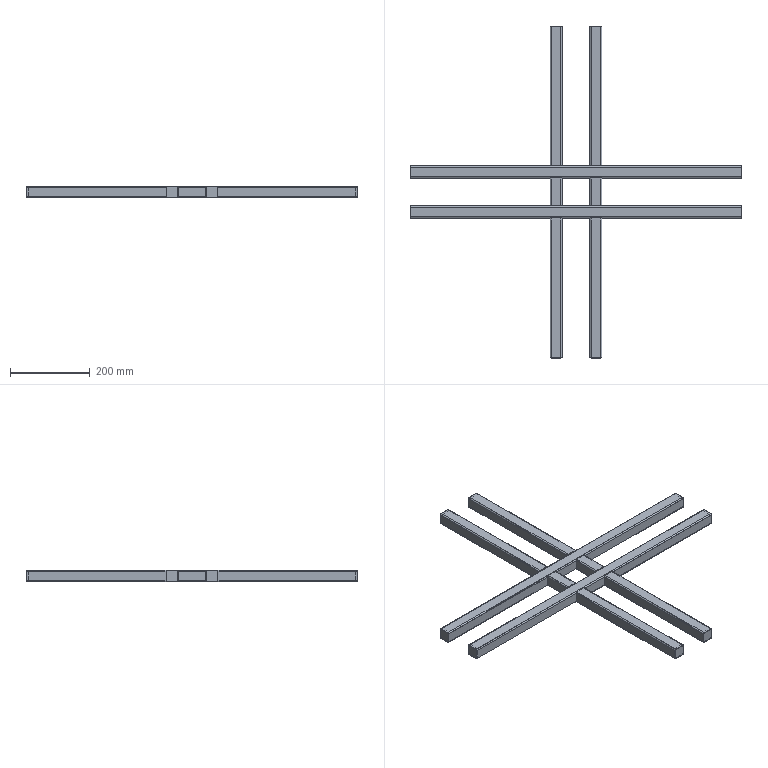Part | SolidWorks | features BaseBody 16 | 16 solids | 224 faces | box 830 x 830 x 30 mm | volume 556865 mm3 | plane 128 | cylinder 96 | commonest cylinder face diameters 6 x64 3 x32